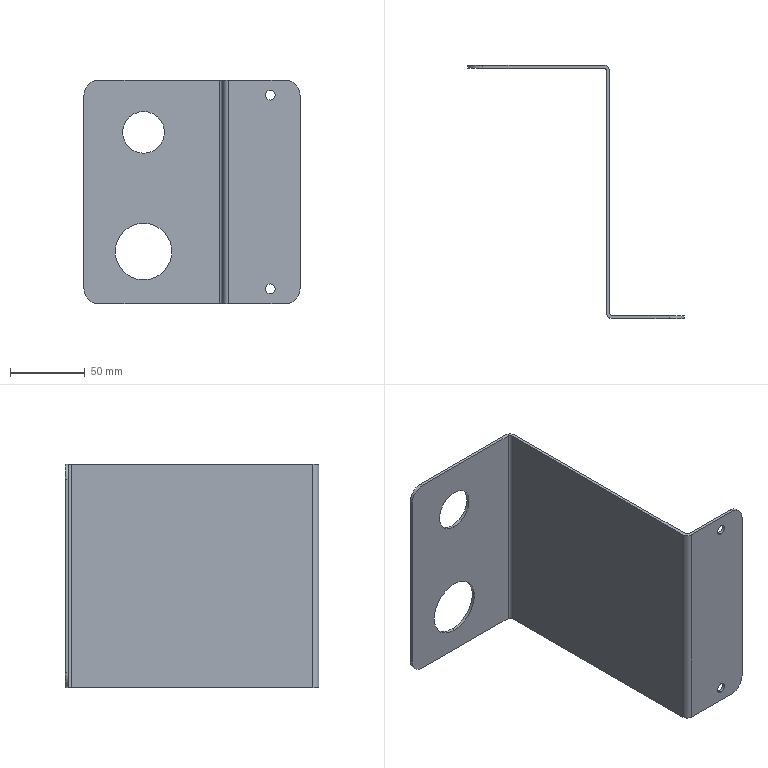Part | SolidWorks | features BaseBody 1 | 1 solid | 26 faces | box 145 x 170 x 150 mm | volume 89319 mm3 | cylinder 16 | plane 10 | commonest cylinder face diameters 6.6 x4 20 x4 4 x2 8 x2 28 x2 38 x2
STEP:
#1=CARTESIAN_POINT('',(30.,-170.,61.7));
#2=VERTEX_POINT('',#1);
#3=CARTESIAN_POINT('',(30.,-170.,68.3));
#4=VERTEX_POINT('',#3);
#5=CARTESIAN_POINT('',(30.,-170.,65.));
#6=DIRECTION('',(0.,1.,0.));
#7=DIRECTION('',(0.,0.,1.));
#8=AXIS2_PLACEMENT_3D('',#5,#6,#7);
#9=CIRCLE('',#8,3.3);
#10=EDGE_CURVE('',#2,#4,#9,.T.);
#11=ORIENTED_EDGE('',*,*,#10,.F.);
#12=CARTESIAN_POINT('',(30.,-168.,61.7));
#13=VERTEX_POINT('',#12);
#14=CARTESIAN_POINT('',(30.,-168.,61.7));
#15=DIRECTION('',(0.,1.,0.));
#16=VECTOR('',#15,1000.);
#17=LINE('',#14,#16);
#18=EDGE_CURVE('',#2,#13,#17,.T.);
#19=ORIENTED_EDGE('',*,*,#18,.T.);
#20=CARTESIAN_POINT('',(30.,-168.,68.3));
#21=VERTEX_POINT('',#20);
#22=CARTESIAN_POINT('',(30.,-168.,65.));
#23=DIRECTION('',(0.,1.,0.));
#24=DIRECTION('',(0.,0.,1.));
#25=AXIS2_PLACEMENT_3D('',#22,#23,#24);
#26=CIRCLE('',#25,3.3);
#27=EDGE_CURVE('',#13,#21,#26,.T.);
#28=ORIENTED_EDGE('',*,*,#27,.T.);
#29=CARTESIAN_POINT('',(30.,-168.,68.3));
#30=DIRECTION('',(0.,1.,0.));
#31=VECTOR('',#30,1000.);
#32=LINE('',#29,#31);
#33=EDGE_CURVE('',#4,#21,#32,.T.);
#34=ORIENTED_EDGE('',*,*,#33,.F.);
#35=EDGE_LOOP('',(#11,#19,#28,#34));
#36=FACE_OUTER_BOUND('',#35,.T.);
#37=CARTESIAN_POINT('',(30.,-168.,65.));
#38=DIRECTION('',(0.,1.,0.));
#39=DIRECTION('',(0.,0.,1.));
#40=AXIS2_PLACEMENT_3D('',#37,#38,#39);
#41=CYLINDRICAL_SURFACE('',#40,3.3);
#42=ADVANCED_FACE('',(#36),#41,.F.);
#43=CARTESIAN_POINT('',(30.,-170.,-68.3));
#44=VERTEX_POINT('',#43);
#45=CARTESIAN_POINT('',(30.,-170.,-61.7));
#46=VERTEX_POINT('',#45);
#47=CARTESIAN_POINT('',(30.,-170.,-65.));
#48=DIRECTION('',(0.,1.,0.));
#49=DIRECTION('',(0.,0.,1.));
#50=AXIS2_PLACEMENT_3D('',#47,#48,#49);
#51=CIRCLE('',#50,3.3);
#52=EDGE_CURVE('',#44,#46,#51,.T.);
#53=ORIENTED_EDGE('',*,*,#52,.F.);
#54=CARTESIAN_POINT('',(30.,-168.,-68.3));
#55=VERTEX_POINT('',#54);
#56=CARTESIAN_POINT('',(30.,-168.,-68.3));
#57=DIRECTION('',(0.,1.,0.));
#58=VECTOR('',#57,1000.);
#59=LINE('',#56,#58);
#60=EDGE_CURVE('',#44,#55,#59,.T.);
#61=ORIENTED_EDGE('',*,*,#60,.T.);
#62=CARTESIAN_POINT('',(30.,-168.,-61.7));
#63=VERTEX_POINT('',#62);
#64=CARTESIAN_POINT('',(30.,-168.,-65.));
#65=DIRECTION('',(0.,1.,0.));
#66=DIRECTION('',(0.,0.,1.));
#67=AXIS2_PLACEMENT_3D('',#64,#65,#66);
#68=CIRCLE('',#67,3.3);
#69=EDGE_CURVE('',#55,#63,#68,.T.);
#70=ORIENTED_EDGE('',*,*,#69,.T.);
#71=CARTESIAN_POINT('',(30.,-168.,-61.7));
#72=DIRECTION('',(0.,1.,0.));
#73=VECTOR('',#72,1000.);
#74=LINE('',#71,#73);
#75=EDGE_CURVE('',#46,#63,#74,.T.);
#76=ORIENTED_EDGE('',*,*,#75,.F.);
#77=EDGE_LOOP('',(#53,#61,#70,#76));
#78=FACE_OUTER_BOUND('',#77,.T.);
#79=CARTESIAN_POINT('',(30.,-168.,-65.));
#80=DIRECTION('',(0.,1.,0.));
#81=DIRECTION('',(0.,0.,1.));
#82=AXIS2_PLACEMENT_3D('',#79,#80,#81);
#83=CYLINDRICAL_SURFACE('',#82,3.3);
#84=ADVANCED_FACE('',(#78),#83,.F.);
#85=CARTESIAN_POINT('',(-55.,-2.,-59.));
#86=VERTEX_POINT('',#85);
#87=CARTESIAN_POINT('',(-55.,-2.,-21.));
#88=VERTEX_POINT('',#87);
#89=CARTESIAN_POINT('',(-55.,-2.,-40.));
#90=DIRECTION('',(0.,1.,0.));
#91=DIRECTION('',(0.,0.,1.));
#92=AXIS2_PLACEMENT_3D('',#89,#90,#91);
#93=CIRCLE('',#92,19.);
#94=EDGE_CURVE('',#86,#88,#93,.T.);
#95=ORIENTED_EDGE('',*,*,#94,.F.);
#96=CARTESIAN_POINT('',(-55.,0.,-59.));
#97=VERTEX_POINT('',#96);
#98=CARTESIAN_POINT('',(-55.,-170.,-59.));
#99=DIRECTION('',(0.,1.,0.));
#100=VECTOR('',#99,1000.);
#101=LINE('',#98,#100);
#102=EDGE_CURVE('',#86,#97,#101,.T.);
#103=ORIENTED_EDGE('',*,*,#102,.T.);
#104=CARTESIAN_POINT('',(-55.,0.,-21.));
#105=VERTEX_POINT('',#104);
#106=CARTESIAN_POINT('',(-55.,0.,-40.));
#107=DIRECTION('',(0.,1.,0.));
#108=DIRECTION('',(0.,0.,1.));
#109=AXIS2_PLACEMENT_3D('',#106,#107,#108);
#110=CIRCLE('',#109,19.);
#111=EDGE_CURVE('',#97,#105,#110,.T.);
#112=ORIENTED_EDGE('',*,*,#111,.T.);
#113=CARTESIAN_POINT('',(-55.,-170.,-21.));
#114=DIRECTION('',(0.,1.,0.));
#115=VECTOR('',#114,1000.);
#116=LINE('',#113,#115);
#117=EDGE_CURVE('',#88,#105,#116,.T.);
#118=ORIENTED_EDGE('',*,*,#117,.F.);
#119=EDGE_LOOP('',(#95,#103,#112,#118));
#120=FACE_OUTER_BOUND('',#119,.T.);
#121=CARTESIAN_POINT('',(-55.,-170.,-40.));
#122=DIRECTION('',(0.,1.,0.));
#123=DIRECTION('',(0.,0.,1.));
#124=AXIS2_PLACEMENT_3D('',#121,#122,#123);
#125=CYLINDRICAL_SURFACE('',#124,19.);
#126=ADVANCED_FACE('',(#120),#125,.F.);
#127=CARTESIAN_POINT('',(-55.,-2.,26.));
#128=VERTEX_POINT('',#127);
#129=CARTESIAN_POINT('',(-55.,-2.,54.));
#130=VERTEX_POINT('',#129);
#131=CARTESIAN_POINT('',(-55.,-2.,40.));
#132=DIRECTION('',(0.,1.,0.));
#133=DIRECTION('',(0.,0.,1.));
#134=AXIS2_PLACEMENT_3D('',#131,#132,#133);
#135=CIRCLE('',#134,14.);
#136=EDGE_CURVE('',#128,#130,#135,.T.);
#137=ORIENTED_EDGE('',*,*,#136,.F.);
#138=CARTESIAN_POINT('',(-55.,0.,26.));
#139=VERTEX_POINT('',#138);
#140=CARTESIAN_POINT('',(-55.,-170.,26.));
#141=DIRECTION('',(0.,1.,0.));
#142=VECTOR('',#141,1000.);
#143=LINE('',#140,#142);
#144=EDGE_CURVE('',#128,#139,#143,.T.);
#145=ORIENTED_EDGE('',*,*,#144,.T.);
#146=CARTESIAN_POINT('',(-55.,0.,54.));
#147=VERTEX_POINT('',#146);
#148=CARTESIAN_POINT('',(-55.,0.,40.));
#149=DIRECTION('',(0.,1.,0.));
#150=DIRECTION('',(0.,0.,1.));
#151=AXIS2_PLACEMENT_3D('',#148,#149,#150);
#152=CIRCLE('',#151,14.);
#153=EDGE_CURVE('',#139,#147,#152,.T.);
#154=ORIENTED_EDGE('',*,*,#153,.T.);
#155=CARTESIAN_POINT('',(-55.,-170.,54.));
#156=DIRECTION('',(0.,1.,0.));
#157=VECTOR('',#156,1000.);
#158=LINE('',#155,#157);
#159=EDGE_CURVE('',#130,#147,#158,.T.);
#160=ORIENTED_EDGE('',*,*,#159,.F.);
#161=EDGE_LOOP('',(#137,#145,#154,#160));
#162=FACE_OUTER_BOUND('',#161,.T.);
#163=CARTESIAN_POINT('',(-55.,-170.,40.));
#164=DIRECTION('',(0.,1.,0.));
#165=DIRECTION('',(0.,0.,1.));
#166=AXIS2_PLACEMENT_3D('',#163,#164,#165);
#167=CYLINDRICAL_SURFACE('',#166,14.);
#168=ADVANCED_FACE('',(#162),#167,.F.);
#169=CARTESIAN_POINT('',(50.,-168.,-65.));
#170=VERTEX_POINT('',#169);
#171=CARTESIAN_POINT('',(40.,-168.,-75.));
#172=VERTEX_POINT('',#171);
#173=CARTESIAN_POINT('',(40.,-168.,-65.));
#174=DIRECTION('',(0.,1.,0.));
#175=DIRECTION('',(0.,0.,1.));
#176=AXIS2_PLACEMENT_3D('',#173,#174,#175);
#177=CIRCLE('',#176,10.);
#178=EDGE_CURVE('',#170,#172,#177,.T.);
#179=ORIENTED_EDGE('',*,*,#178,.F.);
#180=CARTESIAN_POINT('',(50.,-170.,-65.));
#181=VERTEX_POINT('',#180);
#182=CARTESIAN_POINT('',(50.,-168.,-65.));
#183=DIRECTION('',(0.,1.,0.));
#184=VECTOR('',#183,1000.);
#185=LINE('',#182,#184);
#186=EDGE_CURVE('',#181,#170,#185,.T.);
#187=ORIENTED_EDGE('',*,*,#186,.F.);
#188=CARTESIAN_POINT('',(40.,-170.,-75.));
#189=VERTEX_POINT('',#188);
#190=CARTESIAN_POINT('',(40.,-170.,-65.));
#191=DIRECTION('',(0.,-1.,0.));
#192=DIRECTION('',(0.,0.,1.));
#193=AXIS2_PLACEMENT_3D('',#190,#191,#192);
#194=CIRCLE('',#193,10.);
#195=EDGE_CURVE('',#189,#181,#194,.T.);
#196=ORIENTED_EDGE('',*,*,#195,.F.);
#197=CARTESIAN_POINT('',(40.,-166.,-75.));
#198=DIRECTION('',(0.,-1.,0.));
#199=VECTOR('',#198,1000.);
#200=LINE('',#197,#199);
#201=EDGE_CURVE('',#172,#189,#200,.T.);
#202=ORIENTED_EDGE('',*,*,#201,.F.);
#203=EDGE_LOOP('',(#179,#187,#196,#202));
#204=FACE_OUTER_BOUND('',#203,.T.);
#205=CARTESIAN_POINT('',(40.,-166.,-65.));
#206=DIRECTION('',(0.,-1.,0.));
#207=DIRECTION('',(0.,0.,-1.));
#208=AXIS2_PLACEMENT_3D('',#205,#206,#207);
#209=CYLINDRICAL_SURFACE('',#208,10.);
#210=ADVANCED_FACE('',(#204),#209,.T.);
#211=CARTESIAN_POINT('',(40.,-168.,75.));
#212=VERTEX_POINT('',#211);
#213=CARTESIAN_POINT('',(50.,-168.,65.));
#214=VERTEX_POINT('',#213);
#215=CARTESIAN_POINT('',(40.,-168.,65.));
#216=DIRECTION('',(0.,1.,0.));
#217=DIRECTION('',(0.,0.,1.));
#218=AXIS2_PLACEMENT_3D('',#215,#216,#217);
#219=CIRCLE('',#218,10.);
#220=EDGE_CURVE('',#212,#214,#219,.T.);
#221=ORIENTED_EDGE('',*,*,#220,.F.);
#222=CARTESIAN_POINT('',(40.,-170.,75.));
#223=VERTEX_POINT('',#222);
#224=CARTESIAN_POINT('',(40.,-166.,75.));
#225=DIRECTION('',(0.,1.,0.));
#226=VECTOR('',#225,1000.);
#227=LINE('',#224,#226);
#228=EDGE_CURVE('',#223,#212,#227,.T.);
#229=ORIENTED_EDGE('',*,*,#228,.F.);
#230=CARTESIAN_POINT('',(50.,-170.,65.));
#231=VERTEX_POINT('',#230);
#232=CARTESIAN_POINT('',(40.,-170.,65.));
#233=DIRECTION('',(0.,-1.,0.));
#234=DIRECTION('',(0.,0.,1.));
#235=AXIS2_PLACEMENT_3D('',#232,#233,#234);
#236=CIRCLE('',#235,10.);
#237=EDGE_CURVE('',#231,#223,#236,.T.);
#238=ORIENTED_EDGE('',*,*,#237,.F.);
#239=CARTESIAN_POINT('',(50.,-168.,65.));
#240=DIRECTION('',(0.,-1.,0.));
#241=VECTOR('',#240,1000.);
#242=LINE('',#239,#241);
#243=EDGE_CURVE('',#214,#231,#242,.T.);
#244=ORIENTED_EDGE('',*,*,#243,.F.);
#245=EDGE_LOOP('',(#221,#229,#238,#244));
#246=FACE_OUTER_BOUND('',#245,.T.);
#247=CARTESIAN_POINT('',(40.,-168.,65.));
#248=DIRECTION('',(0.,-1.,0.));
#249=DIRECTION('',(0.,0.,-1.));
#250=AXIS2_PLACEMENT_3D('',#247,#248,#249);
#251=CYLINDRICAL_SURFACE('',#250,10.);
#252=ADVANCED_FACE('',(#246),#251,.T.);
#253=CARTESIAN_POINT('',(-85.,-2.,75.));
#254=VERTEX_POINT('',#253);
#255=CARTESIAN_POINT('',(-95.,-2.,65.));
#256=VERTEX_POINT('',#255);
#257=CARTESIAN_POINT('',(-85.,-2.,65.));
#258=DIRECTION('',(0.,-1.,0.));
#259=DIRECTION('',(0.,0.,1.));
#260=AXIS2_PLACEMENT_3D('',#257,#258,#259);
#261=CIRCLE('',#260,10.);
#262=EDGE_CURVE('',#254,#256,#261,.T.);
#263=ORIENTED_EDGE('',*,*,#262,.F.);
#264=CARTESIAN_POINT('',(-85.,0.,75.));
#265=VERTEX_POINT('',#264);
#266=CARTESIAN_POINT('',(-85.,-2.,75.));
#267=DIRECTION('',(0.,-1.,0.));
#268=VECTOR('',#267,1000.);
#269=LINE('',#266,#268);
#270=EDGE_CURVE('',#265,#254,#269,.T.);
#271=ORIENTED_EDGE('',*,*,#270,.F.);
#272=CARTESIAN_POINT('',(-95.,0.,65.));
#273=VERTEX_POINT('',#272);
#274=CARTESIAN_POINT('',(-85.,0.,65.));
#275=DIRECTION('',(0.,1.,0.));
#276=DIRECTION('',(0.,0.,1.));
#277=AXIS2_PLACEMENT_3D('',#274,#275,#276);
#278=CIRCLE('',#277,10.);
#279=EDGE_CURVE('',#273,#265,#278,.T.);
#280=ORIENTED_EDGE('',*,*,#279,.F.);
#281=CARTESIAN_POINT('',(-95.,0.,65.));
#282=DIRECTION('',(0.,1.,0.));
#283=VECTOR('',#282,1000.);
#284=LINE('',#281,#283);
#285=EDGE_CURVE('',#256,#273,#284,.T.);
#286=ORIENTED_EDGE('',*,*,#285,.F.);
#287=EDGE_LOOP('',(#263,#271,#280,#286));
#288=FACE_OUTER_BOUND('',#287,.T.);
#289=CARTESIAN_POINT('',(-85.,-2.,65.));
#290=DIRECTION('',(0.,-1.,0.));
#291=DIRECTION('',(0.,0.,-1.));
#292=AXIS2_PLACEMENT_3D('',#289,#290,#291);
#293=CYLINDRICAL_SURFACE('',#292,10.);
#294=ADVANCED_FACE('',(#288),#293,.T.);
#295=CARTESIAN_POINT('',(-95.,-2.,-65.));
#296=VERTEX_POINT('',#295);
#297=CARTESIAN_POINT('',(-85.,-2.,-75.));
#298=VERTEX_POINT('',#297);
#299=CARTESIAN_POINT('',(-85.,-2.,-65.));
#300=DIRECTION('',(0.,-1.,0.));
#301=DIRECTION('',(0.,0.,1.));
#302=AXIS2_PLACEMENT_3D('',#299,#300,#301);
#303=CIRCLE('',#302,10.);
#304=EDGE_CURVE('',#296,#298,#303,.T.);
#305=ORIENTED_EDGE('',*,*,#304,.F.);
#306=CARTESIAN_POINT('',(-95.,0.,-65.));
#307=VERTEX_POINT('',#306);
#308=CARTESIAN_POINT('',(-95.,-2.,-65.));
#309=DIRECTION('',(0.,-1.,0.));
#310=VECTOR('',#309,1000.);
#311=LINE('',#308,#310);
#312=EDGE_CURVE('',#307,#296,#311,.T.);
#313=ORIENTED_EDGE('',*,*,#312,.F.);
#314=CARTESIAN_POINT('',(-85.,0.,-75.));
#315=VERTEX_POINT('',#314);
#316=CARTESIAN_POINT('',(-85.,0.,-65.));
#317=DIRECTION('',(0.,1.,0.));
#318=DIRECTION('',(0.,0.,1.));
#319=AXIS2_PLACEMENT_3D('',#316,#317,#318);
#320=CIRCLE('',#319,10.);
#321=EDGE_CURVE('',#315,#307,#320,.T.);
#322=ORIENTED_EDGE('',*,*,#321,.F.);
#323=CARTESIAN_POINT('',(-85.,-4.,-75.));
#324=DIRECTION('',(0.,1.,0.));
#325=VECTOR('',#324,1000.);
#326=LINE('',#323,#325);
#327=EDGE_CURVE('',#298,#315,#326,.T.);
#328=ORIENTED_EDGE('',*,*,#327,.F.);
#329=EDGE_LOOP('',(#305,#313,#322,#328));
#330=FACE_OUTER_BOUND('',#329,.T.);
#331=CARTESIAN_POINT('',(-85.,-4.,-65.));
#332=DIRECTION('',(0.,1.,0.));
#333=DIRECTION('',(0.,0.,1.));
#334=AXIS2_PLACEMENT_3D('',#331,#332,#333);
#335=CYLINDRICAL_SURFACE('',#334,10.);
#336=ADVANCED_FACE('',(#330),#335,.T.);
#337=CARTESIAN_POINT('',(-2.,-166.,-75.));
#338=VERTEX_POINT('',#337);
#339=CARTESIAN_POINT('',(2.,-170.,-75.));
#340=VERTEX_POINT('',#339);
#341=CARTESIAN_POINT('',(2.,-166.,-75.));
#342=DIRECTION('',(0.,0.,1.));
#343=DIRECTION('',(1.,0.,0.));
#344=AXIS2_PLACEMENT_3D('',#341,#342,#343);
#345=CIRCLE('',#344,4.);
#346=EDGE_CURVE('',#338,#340,#345,.T.);
#347=ORIENTED_EDGE('',*,*,#346,.T.);
#348=CARTESIAN_POINT('',(2.,-170.,75.));
#349=VERTEX_POINT('',#348);
#350=CARTESIAN_POINT('',(2.,-170.,75.));
#351=DIRECTION('',(0.,0.,-1.));
#352=VECTOR('',#351,1000.);
#353=LINE('',#350,#352);
#354=EDGE_CURVE('',#349,#340,#353,.T.);
#355=ORIENTED_EDGE('',*,*,#354,.F.);
#356=CARTESIAN_POINT('',(-2.,-166.,75.));
#357=VERTEX_POINT('',#356);
#358=CARTESIAN_POINT('',(2.,-166.,75.));
#359=DIRECTION('',(0.,0.,1.));
#360=DIRECTION('',(1.,0.,0.));
#361=AXIS2_PLACEMENT_3D('',#358,#359,#360);
#362=CIRCLE('',#361,4.);
#363=EDGE_CURVE('',#357,#349,#362,.T.);
#364=ORIENTED_EDGE('',*,*,#363,.F.);
#365=CARTESIAN_POINT('',(-2.,-166.,75.));
#366=DIRECTION('',(0.,0.,-1.));
#367=VECTOR('',#366,1000.);
#368=LINE('',#365,#367);
#369=EDGE_CURVE('',#357,#338,#368,.T.);
#370=ORIENTED_EDGE('',*,*,#369,.T.);
#371=EDGE_LOOP('',(#347,#355,#364,#370));
#372=FACE_OUTER_BOUND('',#371,.T.);
#373=CARTESIAN_POINT('',(2.,-166.,75.));
#374=DIRECTION('',(0.,0.,-1.));
#375=DIRECTION('',(-1.,0.,0.));
#376=AXIS2_PLACEMENT_3D('',#373,#374,#375);
#377=CYLINDRICAL_SURFACE('',#376,4.);
#378=ADVANCED_FACE('',(#372),#377,.T.);
#379=CARTESIAN_POINT('',(-2.,-4.,-75.));
#380=VERTEX_POINT('',#379);
#381=CARTESIAN_POINT('',(-2.,0.,-75.));
#382=DIRECTION('',(0.,-1.,0.));
#383=VECTOR('',#382,1000.);
#384=LINE('',#381,#383);
#385=EDGE_CURVE('',#380,#338,#384,.T.);
#386=ORIENTED_EDGE('',*,*,#385,.T.);
#387=ORIENTED_EDGE('',*,*,#369,.F.);
#388=CARTESIAN_POINT('',(-2.,-4.,75.));
#389=VERTEX_POINT('',#388);
#390=CARTESIAN_POINT('',(-2.,0.,75.));
#391=DIRECTION('',(0.,-1.,0.));
#392=VECTOR('',#391,1000.);
#393=LINE('',#390,#392);
#394=EDGE_CURVE('',#389,#357,#393,.T.);
#395=ORIENTED_EDGE('',*,*,#394,.F.);
#396=CARTESIAN_POINT('',(-2.,-4.,75.));
#397=DIRECTION('',(0.,0.,-1.));
#398=VECTOR('',#397,1000.);
#399=LINE('',#396,#398);
#400=EDGE_CURVE('',#389,#380,#399,.T.);
#401=ORIENTED_EDGE('',*,*,#400,.T.);
#402=EDGE_LOOP('',(#386,#387,#395,#401));
#403=FACE_OUTER_BOUND('',#402,.T.);
#404=CARTESIAN_POINT('',(-2.,0.,75.));
#405=DIRECTION('',(1.,0.,0.));
#406=DIRECTION('',(0.,1.,0.));
#407=AXIS2_PLACEMENT_3D('',#404,#405,#406);
#408=PLANE('',#407);
#409=ADVANCED_FACE('',(#403),#408,.F.);
#410=CARTESIAN_POINT('',(-4.,-2.,-75.));
#411=VERTEX_POINT('',#410);
#412=CARTESIAN_POINT('',(-4.,-4.,-75.));
#413=DIRECTION('',(0.,0.,-1.));
#414=DIRECTION('',(1.,0.,0.));
#415=AXIS2_PLACEMENT_3D('',#412,#413,#414);
#416=CIRCLE('',#415,2.);
#417=EDGE_CURVE('',#411,#380,#416,.T.);
#418=ORIENTED_EDGE('',*,*,#417,.T.);
#419=ORIENTED_EDGE('',*,*,#400,.F.);
#420=CARTESIAN_POINT('',(-4.,-2.,75.));
#421=VERTEX_POINT('',#420);
#422=CARTESIAN_POINT('',(-4.,-4.,75.));
#423=DIRECTION('',(0.,0.,-1.));
#424=DIRECTION('',(1.,0.,0.));
#425=AXIS2_PLACEMENT_3D('',#422,#423,#424);
#426=CIRCLE('',#425,2.);
#427=EDGE_CURVE('',#421,#389,#426,.T.);
#428=ORIENTED_EDGE('',*,*,#427,.F.);
#429=CARTESIAN_POINT('',(-4.,-2.,75.));
#430=DIRECTION('',(0.,0.,-1.));
#431=VECTOR('',#430,1000.);
#432=LINE('',#429,#431);
#433=EDGE_CURVE('',#421,#411,#432,.T.);
#434=ORIENTED_EDGE('',*,*,#433,.T.);
#435=EDGE_LOOP('',(#418,#419,#428,#434));
#436=FACE_OUTER_BOUND('',#435,.T.);
#437=CARTESIAN_POINT('',(-4.,-4.,75.));
#438=DIRECTION('',(0.,0.,-1.));
#439=DIRECTION('',(-1.,0.,0.));
#440=AXIS2_PLACEMENT_3D('',#437,#438,#439);
#441=CYLINDRICAL_SURFACE('',#440,2.);
#442=ADVANCED_FACE('',(#436),#441,.F.);
#443=CARTESIAN_POINT('',(-55.,-2.,40.));
#444=DIRECTION('',(0.,1.,0.));
#445=DIRECTION('',(0.,0.,1.));
#446=AXIS2_PLACEMENT_3D('',#443,#444,#445);
#447=CIRCLE('',#446,14.);
#448=EDGE_CURVE('',#130,#128,#447,.T.);
#449=ORIENTED_EDGE('',*,*,#448,.T.);
#450=ORIENTED_EDGE('',*,*,#136,.T.);
#451=EDGE_LOOP('',(#449,#450));
#452=FACE_BOUND('',#451,.T.);
#453=CARTESIAN_POINT('',(-55.,-2.,-40.));
#454=DIRECTION('',(0.,1.,0.));
#455=DIRECTION('',(0.,0.,1.));
#456=AXIS2_PLACEMENT_3D('',#453,#454,#455);
#457=CIRCLE('',#456,19.);
#458=EDGE_CURVE('',#88,#86,#457,.T.);
#459=ORIENTED_EDGE('',*,*,#458,.T.);
#460=ORIENTED_EDGE('',*,*,#94,.T.);
#461=EDGE_LOOP('',(#459,#460));
#462=FACE_BOUND('',#461,.T.);
#463=CARTESIAN_POINT('',(-95.,-2.,75.));
#464=DIRECTION('',(0.,0.,-1.));
#465=VECTOR('',#464,1000.);
#466=LINE('',#463,#465);
#467=EDGE_CURVE('',#256,#296,#466,.T.);
#468=ORIENTED_EDGE('',*,*,#467,.T.);
#469=ORIENTED_EDGE('',*,*,#304,.T.);
#470=CARTESIAN_POINT('',(-95.,-2.,-75.));
#471=DIRECTION('',(1.,0.,0.));
#472=VECTOR('',#471,1000.);
#473=LINE('',#470,#472);
#474=EDGE_CURVE('',#298,#411,#473,.T.);
#475=ORIENTED_EDGE('',*,*,#474,.T.);
#476=ORIENTED_EDGE('',*,*,#433,.F.);
#477=CARTESIAN_POINT('',(-95.,-2.,75.));
#478=DIRECTION('',(1.,0.,0.));
#479=VECTOR('',#478,1000.);
#480=LINE('',#477,#479);
#481=EDGE_CURVE('',#254,#421,#480,.T.);
#482=ORIENTED_EDGE('',*,*,#481,.F.);
#483=ORIENTED_EDGE('',*,*,#262,.T.);
#484=EDGE_LOOP('',(#468,#469,#475,#476,#482,#483));
#485=FACE_OUTER_BOUND('',#484,.T.);
#486=CARTESIAN_POINT('',(-95.,-2.,75.));
#487=DIRECTION('',(0.,1.,0.));
#488=DIRECTION('',(1.,0.,0.));
#489=AXIS2_PLACEMENT_3D('',#486,#487,#488);
#490=PLANE('',#489);
#491=ADVANCED_FACE('',(#452,#462,#485),#490,.F.);
#492=CARTESIAN_POINT('',(-95.,0.,75.));
#493=DIRECTION('',(0.,0.,-1.));
#494=VECTOR('',#493,1000.);
#495=LINE('',#492,#494);
#496=EDGE_CURVE('',#273,#307,#495,.T.);
#497=ORIENTED_EDGE('',*,*,#496,.T.);
#498=ORIENTED_EDGE('',*,*,#312,.T.);
#499=ORIENTED_EDGE('',*,*,#467,.F.);
#500=ORIENTED_EDGE('',*,*,#285,.T.);
#501=EDGE_LOOP('',(#497,#498,#499,#500));
#502=FACE_OUTER_BOUND('',#501,.T.);
#503=CARTESIAN_POINT('',(-95.,-2.,75.));
#504=DIRECTION('',(-1.,0.,0.));
#505=DIRECTION('',(0.,0.,1.));
#506=AXIS2_PLACEMENT_3D('',#503,#504,#505);
#507=PLANE('',#506);
#508=ADVANCED_FACE('',(#502),#507,.T.);
#509=CARTESIAN_POINT('',(-55.,0.,40.));
#510=DIRECTION('',(0.,1.,0.));
#511=DIRECTION('',(0.,0.,1.));
#512=AXIS2_PLACEMENT_3D('',#509,#510,#511);
#513=CIRCLE('',#512,14.);
#514=EDGE_CURVE('',#147,#139,#513,.T.);
#515=ORIENTED_EDGE('',*,*,#514,.F.);
#516=ORIENTED_EDGE('',*,*,#153,.F.);
#517=EDGE_LOOP('',(#515,#516));
#518=FACE_BOUND('',#517,.T.);
#519=CARTESIAN_POINT('',(-55.,0.,-40.));
#520=DIRECTION('',(0.,1.,0.));
#521=DIRECTION('',(0.,0.,1.));
#522=AXIS2_PLACEMENT_3D('',#519,#520,#521);
#523=CIRCLE('',#522,19.);
#524=EDGE_CURVE('',#105,#97,#523,.T.);
#525=ORIENTED_EDGE('',*,*,#524,.F.);
#526=ORIENTED_EDGE('',*,*,#111,.F.);
#527=EDGE_LOOP('',(#525,#526));
#528=FACE_BOUND('',#527,.T.);
#529=CARTESIAN_POINT('',(-4.,0.,-75.));
#530=VERTEX_POINT('',#529);
#531=CARTESIAN_POINT('',(-95.,0.,-75.));
#532=DIRECTION('',(1.,0.,0.));
#533=VECTOR('',#532,1000.);
#534=LINE('',#531,#533);
#535=EDGE_CURVE('',#315,#530,#534,.T.);
#536=ORIENTED_EDGE('',*,*,#535,.F.);
#537=ORIENTED_EDGE('',*,*,#321,.T.);
#538=ORIENTED_EDGE('',*,*,#496,.F.);
#539=ORIENTED_EDGE('',*,*,#279,.T.);
#540=CARTESIAN_POINT('',(-4.,0.,75.));
#541=VERTEX_POINT('',#540);
#542=CARTESIAN_POINT('',(-95.,0.,75.));
#543=DIRECTION('',(1.,0.,0.));
#544=VECTOR('',#543,1000.);
#545=LINE('',#542,#544);
#546=EDGE_CURVE('',#265,#541,#545,.T.);
#547=ORIENTED_EDGE('',*,*,#546,.T.);
#548=CARTESIAN_POINT('',(-4.,0.,75.));
#549=DIRECTION('',(0.,0.,-1.));
#550=VECTOR('',#549,1000.);
#551=LINE('',#548,#550);
#552=EDGE_CURVE('',#541,#530,#551,.T.);
#553=ORIENTED_EDGE('',*,*,#552,.T.);
#554=EDGE_LOOP('',(#536,#537,#538,#539,#547,#553));
#555=FACE_OUTER_BOUND('',#554,.T.);
#556=CARTESIAN_POINT('',(-95.,0.,75.));
#557=DIRECTION('',(0.,1.,0.));
#558=DIRECTION('',(1.,0.,0.));
#559=AXIS2_PLACEMENT_3D('',#556,#557,#558);
#560=PLANE('',#559);
#561=ADVANCED_FACE('',(#518,#528,#555),#560,.T.);
#562=CARTESIAN_POINT('',(0.,-4.,-75.));
#563=VERTEX_POINT('',#562);
#564=CARTESIAN_POINT('',(-4.,-4.,-75.));
#565=DIRECTION('',(0.,0.,-1.));
#566=DIRECTION('',(1.,0.,0.));
#567=AXIS2_PLACEMENT_3D('',#564,#565,#566);
#568=CIRCLE('',#567,4.);
#569=EDGE_CURVE('',#530,#563,#568,.T.);
#570=ORIENTED_EDGE('',*,*,#569,.F.);
#571=ORIENTED_EDGE('',*,*,#552,.F.);
#572=CARTESIAN_POINT('',(0.,-4.,75.));
#573=VERTEX_POINT('',#572);
#574=CARTESIAN_POINT('',(-4.,-4.,75.));
#575=DIRECTION('',(0.,0.,-1.));
#576=DIRECTION('',(1.,0.,0.));
#577=AXIS2_PLACEMENT_3D('',#574,#575,#576);
#578=CIRCLE('',#577,4.);
#579=EDGE_CURVE('',#541,#573,#578,.T.);
#580=ORIENTED_EDGE('',*,*,#579,.T.);
#581=CARTESIAN_POINT('',(0.,-4.,75.));
#582=DIRECTION('',(0.,0.,-1.));
#583=VECTOR('',#582,1000.);
#584=LINE('',#581,#583);
#585=EDGE_CURVE('',#573,#563,#584,.T.);
#586=ORIENTED_EDGE('',*,*,#585,.T.);
#587=EDGE_LOOP('',(#570,#571,#580,#586));
#588=FACE_OUTER_BOUND('',#587,.T.);
#589=CARTESIAN_POINT('',(-4.,-4.,75.));
#590=DIRECTION('',(0.,0.,-1.));
#591=DIRECTION('',(-1.,0.,0.));
#592=AXIS2_PLACEMENT_3D('',#589,#590,#591);
#593=CYLINDRICAL_SURFACE('',#592,4.);
#594=ADVANCED_FACE('',(#588),#593,.T.);
#595=CARTESIAN_POINT('',(0.,-166.,-75.));
#596=VERTEX_POINT('',#595);
#597=CARTESIAN_POINT('',(0.,0.,-75.));
#598=DIRECTION('',(0.,-1.,0.));
#599=VECTOR('',#598,1000.);
#600=LINE('',#597,#599);
#601=EDGE_CURVE('',#563,#596,#600,.T.);
#602=ORIENTED_EDGE('',*,*,#601,.F.);
#603=ORIENTED_EDGE('',*,*,#585,.F.);
#604=CARTESIAN_POINT('',(0.,-166.,75.));
#605=VERTEX_POINT('',#604);
#606=CARTESIAN_POINT('',(0.,0.,75.));
#607=DIRECTION('',(0.,-1.,0.));
#608=VECTOR('',#607,1000.);
#609=LINE('',#606,#608);
#610=EDGE_CURVE('',#573,#605,#609,.T.);
#611=ORIENTED_EDGE('',*,*,#610,.T.);
#612=CARTESIAN_POINT('',(0.,-166.,75.));
#613=DIRECTION('',(0.,0.,-1.));
#614=VECTOR('',#613,1000.);
#615=LINE('',#612,#614);
#616=EDGE_CURVE('',#605,#596,#615,.T.);
#617=ORIENTED_EDGE('',*,*,#616,.T.);
#618=EDGE_LOOP('',(#602,#603,#611,#617));
#619=FACE_OUTER_BOUND('',#618,.T.);
#620=CARTESIAN_POINT('',(0.,0.,75.));
#621=DIRECTION('',(1.,0.,0.));
#622=DIRECTION('',(0.,1.,0.));
#623=AXIS2_PLACEMENT_3D('',#620,#621,#622);
#624=PLANE('',#623);
#625=ADVANCED_FACE('',(#619),#624,.T.);
#626=CARTESIAN_POINT('',(2.,-168.,-75.));
#627=VERTEX_POINT('',#626);
#628=CARTESIAN_POINT('',(2.,-166.,-75.));
#629=DIRECTION('',(0.,0.,1.));
#630=DIRECTION('',(-1.,0.,0.));
#631=AXIS2_PLACEMENT_3D('',#628,#629,#630);
#632=CIRCLE('',#631,2.);
#633=EDGE_CURVE('',#596,#627,#632,.T.);
#634=ORIENTED_EDGE('',*,*,#633,.F.);
#635=ORIENTED_EDGE('',*,*,#616,.F.);
#636=CARTESIAN_POINT('',(2.,-168.,75.));
#637=VERTEX_POINT('',#636);
#638=CARTESIAN_POINT('',(2.,-166.,75.));
#639=DIRECTION('',(0.,0.,1.));
#640=DIRECTION('',(-1.,0.,0.));
#641=AXIS2_PLACEMENT_3D('',#638,#639,#640);
#642=CIRCLE('',#641,2.);
#643=EDGE_CURVE('',#605,#637,#642,.T.);
#644=ORIENTED_EDGE('',*,*,#643,.T.);
#645=CARTESIAN_POINT('',(2.,-168.,75.));
#646=DIRECTION('',(0.,0.,-1.));
#647=VECTOR('',#646,1000.);
#648=LINE('',#645,#647);
#649=EDGE_CURVE('',#637,#627,#648,.T.);
#650=ORIENTED_EDGE('',*,*,#649,.T.);
#651=EDGE_LOOP('',(#634,#635,#644,#650));
#652=FACE_OUTER_BOUND('',#651,.T.);
#653=CARTESIAN_POINT('',(2.,-166.,75.));
#654=DIRECTION('',(0.,0.,-1.));
#655=DIRECTION('',(-1.,0.,0.));
#656=AXIS2_PLACEMENT_3D('',#653,#654,#655);
#657=CYLINDRICAL_SURFACE('',#656,2.);
#658=ADVANCED_FACE('',(#652),#657,.F.);
#659=CARTESIAN_POINT('',(30.,-168.,-65.));
#660=DIRECTION('',(0.,1.,0.));
#661=DIRECTION('',(0.,0.,1.));
#662=AXIS2_PLACEMENT_3D('',#659,#660,#661);
#663=CIRCLE('',#662,3.3);
#664=EDGE_CURVE('',#63,#55,#663,.T.);
#665=ORIENTED_EDGE('',*,*,#664,.F.);
#666=ORIENTED_EDGE('',*,*,#69,.F.);
#667=EDGE_LOOP('',(#665,#666));
#668=FACE_BOUND('',#667,.T.);
#669=CARTESIAN_POINT('',(30.,-168.,65.));
#670=DIRECTION('',(0.,1.,0.));
#671=DIRECTION('',(0.,0.,1.));
#672=AXIS2_PLACEMENT_3D('',#669,#670,#671);
#673=CIRCLE('',#672,3.3);
#674=EDGE_CURVE('',#21,#13,#673,.T.);
#675=ORIENTED_EDGE('',*,*,#674,.F.);
#676=ORIENTED_EDGE('',*,*,#27,.F.);
#677=EDGE_LOOP('',(#675,#676));
#678=FACE_BOUND('',#677,.T.);
#679=CARTESIAN_POINT('',(0.,-168.,75.));
#680=DIRECTION('',(1.,0.,0.));
#681=VECTOR('',#680,1000.);
#682=LINE('',#679,#681);
#683=EDGE_CURVE('',#637,#212,#682,.T.);
#684=ORIENTED_EDGE('',*,*,#683,.T.);
#685=ORIENTED_EDGE('',*,*,#220,.T.);
#686=CARTESIAN_POINT('',(50.,-168.,75.));
#687=DIRECTION('',(0.,0.,-1.));
#688=VECTOR('',#687,1000.);
#689=LINE('',#686,#688);
#690=EDGE_CURVE('',#214,#170,#689,.T.);
#691=ORIENTED_EDGE('',*,*,#690,.T.);
#692=ORIENTED_EDGE('',*,*,#178,.T.);
#693=CARTESIAN_POINT('',(0.,-168.,-75.));
#694=DIRECTION('',(1.,0.,0.));
#695=VECTOR('',#694,1000.);
#696=LINE('',#693,#695);
#697=EDGE_CURVE('',#627,#172,#696,.T.);
#698=ORIENTED_EDGE('',*,*,#697,.F.);
#699=ORIENTED_EDGE('',*,*,#649,.F.);
#700=EDGE_LOOP('',(#684,#685,#691,#692,#698,#699));
#701=FACE_OUTER_BOUND('',#700,.T.);
#702=CARTESIAN_POINT('',(0.,-168.,75.));
#703=DIRECTION('',(0.,1.,0.));
#704=DIRECTION('',(1.,0.,0.));
#705=AXIS2_PLACEMENT_3D('',#702,#703,#704);
#706=PLANE('',#705);
#707=ADVANCED_FACE('',(#668,#678,#701),#706,.T.);
#708=ORIENTED_EDGE('',*,*,#690,.F.);
#709=ORIENTED_EDGE('',*,*,#243,.T.);
#710=CARTESIAN_POINT('',(50.,-170.,75.));
#711=DIRECTION('',(0.,0.,-1.));
#712=VECTOR('',#711,1000.);
#713=LINE('',#710,#712);
#714=EDGE_CURVE('',#231,#181,#713,.T.);
#715=ORIENTED_EDGE('',*,*,#714,.T.);
#716=ORIENTED_EDGE('',*,*,#186,.T.);
#717=EDGE_LOOP('',(#708,#709,#715,#716));
#718=FACE_OUTER_BOUND('',#717,.T.);
#719=CARTESIAN_POINT('',(50.,-168.,75.));
#720=DIRECTION('',(1.,0.,0.));
#721=DIRECTION('',(0.,1.,0.));
#722=AXIS2_PLACEMENT_3D('',#719,#720,#721);
#723=PLANE('',#722);
#724=ADVANCED_FACE('',(#718),#723,.T.);
#725=CARTESIAN_POINT('',(30.,-170.,-65.));
#726=DIRECTION('',(0.,1.,0.));
#727=DIRECTION('',(0.,0.,1.));
#728=AXIS2_PLACEMENT_3D('',#725,#726,#727);
#729=CIRCLE('',#728,3.3);
#730=EDGE_CURVE('',#46,#44,#729,.T.);
#731=ORIENTED_EDGE('',*,*,#730,.T.);
#732=ORIENTED_EDGE('',*,*,#52,.T.);
#733=EDGE_LOOP('',(#731,#732));
#734=FACE_BOUND('',#733,.T.);
#735=CARTESIAN_POINT('',(30.,-170.,65.));
#736=DIRECTION('',(0.,1.,0.));
#737=DIRECTION('',(0.,0.,1.));
#738=AXIS2_PLACEMENT_3D('',#735,#736,#737);
#739=CIRCLE('',#738,3.3);
#740=EDGE_CURVE('',#4,#2,#739,.T.);
#741=ORIENTED_EDGE('',*,*,#740,.T.);
#742=ORIENTED_EDGE('',*,*,#10,.T.);
#743=EDGE_LOOP('',(#741,#742));
#744=FACE_BOUND('',#743,.T.);
#745=ORIENTED_EDGE('',*,*,#714,.F.);
#746=ORIENTED_EDGE('',*,*,#237,.T.);
#747=CARTESIAN_POINT('',(0.,-170.,75.));
#748=DIRECTION('',(1.,0.,0.));
#749=VECTOR('',#748,1000.);
#750=LINE('',#747,#749);
#751=EDGE_CURVE('',#349,#223,#750,.T.);
#752=ORIENTED_EDGE('',*,*,#751,.F.);
#753=ORIENTED_EDGE('',*,*,#354,.T.);
#754=CARTESIAN_POINT('',(0.,-170.,-75.));
#755=DIRECTION('',(1.,0.,0.));
#756=VECTOR('',#755,1000.);
#757=LINE('',#754,#756);
#758=EDGE_CURVE('',#340,#189,#757,.T.);
#759=ORIENTED_EDGE('',*,*,#758,.T.);
#760=ORIENTED_EDGE('',*,*,#195,.T.);
#761=EDGE_LOOP('',(#745,#746,#752,#753,#759,#760));
#762=FACE_OUTER_BOUND('',#761,.T.);
#763=CARTESIAN_POINT('',(0.,-170.,75.));
#764=DIRECTION('',(0.,1.,0.));
#765=DIRECTION('',(1.,0.,0.));
#766=AXIS2_PLACEMENT_3D('',#763,#764,#765);
#767=PLANE('',#766);
#768=ADVANCED_FACE('',(#734,#744,#762),#767,.F.);
#769=ORIENTED_EDGE('',*,*,#417,.F.);
#770=ORIENTED_EDGE('',*,*,#474,.F.);
#771=ORIENTED_EDGE('',*,*,#327,.T.);
#772=ORIENTED_EDGE('',*,*,#535,.T.);
#773=ORIENTED_EDGE('',*,*,#569,.T.);
#774=ORIENTED_EDGE('',*,*,#601,.T.);
#775=ORIENTED_EDGE('',*,*,#633,.T.);
#776=ORIENTED_EDGE('',*,*,#697,.T.);
#777=ORIENTED_EDGE('',*,*,#201,.T.);
#778=ORIENTED_EDGE('',*,*,#758,.F.);
#779=ORIENTED_EDGE('',*,*,#346,.F.);
#780=ORIENTED_EDGE('',*,*,#385,.F.);
#781=EDGE_LOOP('',(#769,#770,#771,#772,#773,#774,#775,#776,#777,#778,#779,#780));
#782=FACE_OUTER_BOUND('',#781,.T.);
#783=CARTESIAN_POINT('',(-4.,0.,-75.));
#784=DIRECTION('',(0.,0.,-1.));
#785=DIRECTION('',(0.,-1.,0.));
#786=AXIS2_PLACEMENT_3D('',#783,#784,#785);
#787=PLANE('',#786);
#788=ADVANCED_FACE('',(#782),#787,.T.);
#789=ORIENTED_EDGE('',*,*,#427,.T.);
#790=ORIENTED_EDGE('',*,*,#394,.T.);
#791=ORIENTED_EDGE('',*,*,#363,.T.);
#792=ORIENTED_EDGE('',*,*,#751,.T.);
#793=ORIENTED_EDGE('',*,*,#228,.T.);
#794=ORIENTED_EDGE('',*,*,#683,.F.);
#795=ORIENTED_EDGE('',*,*,#643,.F.);
#796=ORIENTED_EDGE('',*,*,#610,.F.);
#797=ORIENTED_EDGE('',*,*,#579,.F.);
#798=ORIENTED_EDGE('',*,*,#546,.F.);
#799=ORIENTED_EDGE('',*,*,#270,.T.);
#800=ORIENTED_EDGE('',*,*,#481,.T.);
#801=EDGE_LOOP('',(#789,#790,#791,#792,#793,#794,#795,#796,#797,#798,#799,#800));
#802=FACE_OUTER_BOUND('',#801,.T.);
#803=CARTESIAN_POINT('',(0.,-4.,75.));
#804=DIRECTION('',(0.,0.,1.));
#805=DIRECTION('',(1.,0.,0.));
#806=AXIS2_PLACEMENT_3D('',#803,#804,#805);
#807=PLANE('',#806);
#808=ADVANCED_FACE('',(#802),#807,.T.);
#809=ORIENTED_EDGE('',*,*,#144,.F.);
#810=ORIENTED_EDGE('',*,*,#448,.F.);
#811=ORIENTED_EDGE('',*,*,#159,.T.);
#812=ORIENTED_EDGE('',*,*,#514,.T.);
#813=EDGE_LOOP('',(#809,#810,#811,#812));
#814=FACE_OUTER_BOUND('',#813,.T.);
#815=CARTESIAN_POINT('',(-55.,-170.,40.));
#816=DIRECTION('',(0.,1.,0.));
#817=DIRECTION('',(0.,0.,1.));
#818=AXIS2_PLACEMENT_3D('',#815,#816,#817);
#819=CYLINDRICAL_SURFACE('',#818,14.);
#820=ADVANCED_FACE('',(#814),#819,.F.);
#821=ORIENTED_EDGE('',*,*,#102,.F.);
#822=ORIENTED_EDGE('',*,*,#458,.F.);
#823=ORIENTED_EDGE('',*,*,#117,.T.);
#824=ORIENTED_EDGE('',*,*,#524,.T.);
#825=EDGE_LOOP('',(#821,#822,#823,#824));
#826=FACE_OUTER_BOUND('',#825,.T.);
#827=CARTESIAN_POINT('',(-55.,-170.,-40.));
#828=DIRECTION('',(0.,1.,0.));
#829=DIRECTION('',(0.,0.,1.));
#830=AXIS2_PLACEMENT_3D('',#827,#828,#829);
#831=CYLINDRICAL_SURFACE('',#830,19.);
#832=ADVANCED_FACE('',(#826),#831,.F.);
#833=ORIENTED_EDGE('',*,*,#60,.F.);
#834=ORIENTED_EDGE('',*,*,#730,.F.);
#835=ORIENTED_EDGE('',*,*,#75,.T.);
#836=ORIENTED_EDGE('',*,*,#664,.T.);
#837=EDGE_LOOP('',(#833,#834,#835,#836));
#838=FACE_OUTER_BOUND('',#837,.T.);
#839=CARTESIAN_POINT('',(30.,-168.,-65.));
#840=DIRECTION('',(0.,1.,0.));
#841=DIRECTION('',(0.,0.,1.));
#842=AXIS2_PLACEMENT_3D('',#839,#840,#841);
#843=CYLINDRICAL_SURFACE('',#842,3.3);
#844=ADVANCED_FACE('',(#838),#843,.F.);
#845=ORIENTED_EDGE('',*,*,#18,.F.);
#846=ORIENTED_EDGE('',*,*,#740,.F.);
#847=ORIENTED_EDGE('',*,*,#33,.T.);
#848=ORIENTED_EDGE('',*,*,#674,.T.);
#849=EDGE_LOOP('',(#845,#846,#847,#848));
#850=FACE_OUTER_BOUND('',#849,.T.);
#851=CARTESIAN_POINT('',(30.,-168.,65.));
#852=DIRECTION('',(0.,1.,0.));
#853=DIRECTION('',(0.,0.,1.));
#854=AXIS2_PLACEMENT_3D('',#851,#852,#853);
#855=CYLINDRICAL_SURFACE('',#854,3.3);
#856=ADVANCED_FACE('',(#850),#855,.F.);
#857=CLOSED_SHELL('',(#42,#84,#126,#168,#210,#252,#294,#336,#378,#409,#442,#491,#508,#561,#594,#625,#658,#707,#724,#768,#788,#808,#820,#832,#844,#856));
#858=MANIFOLD_SOLID_BREP('',#857);
#859=CARTESIAN_POINT('',(0.,0.,0.));
#860=DIRECTION('',(0.,0.,1.));
#861=DIRECTION('',(1.,0.,0.));
#862=AXIS2_PLACEMENT_3D('',#859,#860,#861);
#863=(LENGTH_UNIT()NAMED_UNIT(*)SI_UNIT(.MILLI.,.METRE.));
#864=UNCERTAINTY_MEASURE_WITH_UNIT(LENGTH_MEASURE(0.00001),#863,'','');
#865=(NAMED_UNIT(*)PLANE_ANGLE_UNIT()SI_UNIT($,.RADIAN.));
#866=(NAMED_UNIT(*)SI_UNIT($,.STERADIAN.)SOLID_ANGLE_UNIT());
#867=(GEOMETRIC_REPRESENTATION_CONTEXT(3)GLOBAL_UNCERTAINTY_ASSIGNED_CONTEXT((#864))GLOBAL_UNIT_ASSIGNED_CONTEXT((#863,#865,#866))REPRESENTATION_CONTEXT('',''));
#868=ADVANCED_BREP_SHAPE_REPRESENTATION('',(#858,#862),#867);